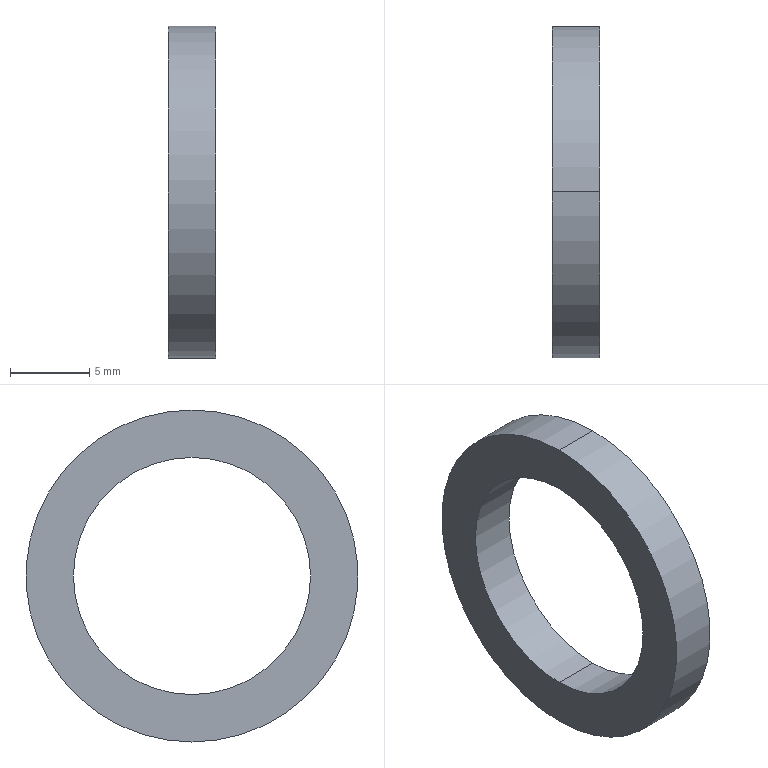Part | SolidWorks | features BaseBody 1 | 1 solid | 6 faces | box 3 x 21 x 21 mm | volume 508.938 mm3 | cylinder 4 | plane 2 | commonest cylinder face diameters 15 x2 21 x2
STEP:
#1=CARTESIAN_POINT('',(3.,0.,10.5));
#2=VERTEX_POINT('',#1);
#3=CARTESIAN_POINT('',(3.,0.,-10.5));
#4=VERTEX_POINT('',#3);
#5=CARTESIAN_POINT('',(3.,0.,0.));
#6=DIRECTION('',(-1.,0.,0.));
#7=DIRECTION('',(0.,0.,1.));
#8=AXIS2_PLACEMENT_3D('',#5,#6,#7);
#9=CIRCLE('',#8,10.5);
#10=EDGE_CURVE('',#2,#4,#9,.T.);
#11=ORIENTED_EDGE('',*,*,#10,.T.);
#12=CARTESIAN_POINT('',(0.,0.,-10.5));
#13=VERTEX_POINT('',#12);
#14=CARTESIAN_POINT('',(3.,0.,-10.5));
#15=DIRECTION('',(-1.,0.,0.));
#16=VECTOR('',#15,1000.);
#17=LINE('',#14,#16);
#18=EDGE_CURVE('',#4,#13,#17,.T.);
#19=ORIENTED_EDGE('',*,*,#18,.T.);
#20=CARTESIAN_POINT('',(0.,0.,10.5));
#21=VERTEX_POINT('',#20);
#22=CARTESIAN_POINT('',(0.,0.,0.));
#23=DIRECTION('',(1.,0.,0.));
#24=DIRECTION('',(0.,0.,1.));
#25=AXIS2_PLACEMENT_3D('',#22,#23,#24);
#26=CIRCLE('',#25,10.5);
#27=EDGE_CURVE('',#13,#21,#26,.T.);
#28=ORIENTED_EDGE('',*,*,#27,.T.);
#29=CARTESIAN_POINT('',(3.,0.,10.5));
#30=DIRECTION('',(-1.,0.,0.));
#31=VECTOR('',#30,1000.);
#32=LINE('',#29,#31);
#33=EDGE_CURVE('',#2,#21,#32,.T.);
#34=ORIENTED_EDGE('',*,*,#33,.F.);
#35=EDGE_LOOP('',(#11,#19,#28,#34));
#36=FACE_OUTER_BOUND('',#35,.T.);
#37=CARTESIAN_POINT('',(3.,0.,0.));
#38=DIRECTION('',(-1.,0.,0.));
#39=DIRECTION('',(0.,0.,1.));
#40=AXIS2_PLACEMENT_3D('',#37,#38,#39);
#41=CYLINDRICAL_SURFACE('',#40,10.5);
#42=ADVANCED_FACE('',(#36),#41,.T.);
#43=CARTESIAN_POINT('',(3.,0.,-7.5));
#44=VERTEX_POINT('',#43);
#45=CARTESIAN_POINT('',(3.,0.,7.5));
#46=VERTEX_POINT('',#45);
#47=CARTESIAN_POINT('',(3.,0.,0.));
#48=DIRECTION('',(-1.,0.,0.));
#49=DIRECTION('',(0.,0.,1.));
#50=AXIS2_PLACEMENT_3D('',#47,#48,#49);
#51=CIRCLE('',#50,7.5);
#52=EDGE_CURVE('',#44,#46,#51,.T.);
#53=ORIENTED_EDGE('',*,*,#52,.F.);
#54=CARTESIAN_POINT('',(0.,0.,-7.5));
#55=VERTEX_POINT('',#54);
#56=CARTESIAN_POINT('',(3.,0.,-7.5));
#57=DIRECTION('',(-1.,0.,0.));
#58=VECTOR('',#57,1000.);
#59=LINE('',#56,#58);
#60=EDGE_CURVE('',#44,#55,#59,.T.);
#61=ORIENTED_EDGE('',*,*,#60,.T.);
#62=CARTESIAN_POINT('',(0.,0.,7.5));
#63=VERTEX_POINT('',#62);
#64=CARTESIAN_POINT('',(0.,0.,0.));
#65=DIRECTION('',(1.,0.,0.));
#66=DIRECTION('',(0.,0.,1.));
#67=AXIS2_PLACEMENT_3D('',#64,#65,#66);
#68=CIRCLE('',#67,7.5);
#69=EDGE_CURVE('',#63,#55,#68,.T.);
#70=ORIENTED_EDGE('',*,*,#69,.F.);
#71=CARTESIAN_POINT('',(3.,0.,7.5));
#72=DIRECTION('',(-1.,0.,0.));
#73=VECTOR('',#72,1000.);
#74=LINE('',#71,#73);
#75=EDGE_CURVE('',#46,#63,#74,.T.);
#76=ORIENTED_EDGE('',*,*,#75,.F.);
#77=EDGE_LOOP('',(#53,#61,#70,#76));
#78=FACE_OUTER_BOUND('',#77,.T.);
#79=CARTESIAN_POINT('',(3.,0.,0.));
#80=DIRECTION('',(-1.,0.,0.));
#81=DIRECTION('',(0.,0.,1.));
#82=AXIS2_PLACEMENT_3D('',#79,#80,#81);
#83=CYLINDRICAL_SURFACE('',#82,7.5);
#84=ADVANCED_FACE('',(#78),#83,.F.);
#85=ORIENTED_EDGE('',*,*,#18,.F.);
#86=CARTESIAN_POINT('',(3.,0.,0.));
#87=DIRECTION('',(-1.,0.,0.));
#88=DIRECTION('',(0.,0.,1.));
#89=AXIS2_PLACEMENT_3D('',#86,#87,#88);
#90=CIRCLE('',#89,10.5);
#91=EDGE_CURVE('',#4,#2,#90,.T.);
#92=ORIENTED_EDGE('',*,*,#91,.T.);
#93=ORIENTED_EDGE('',*,*,#33,.T.);
#94=CARTESIAN_POINT('',(0.,0.,0.));
#95=DIRECTION('',(1.,0.,0.));
#96=DIRECTION('',(0.,0.,1.));
#97=AXIS2_PLACEMENT_3D('',#94,#95,#96);
#98=CIRCLE('',#97,10.5);
#99=EDGE_CURVE('',#21,#13,#98,.T.);
#100=ORIENTED_EDGE('',*,*,#99,.T.);
#101=EDGE_LOOP('',(#85,#92,#93,#100));
#102=FACE_OUTER_BOUND('',#101,.T.);
#103=CARTESIAN_POINT('',(3.,0.,0.));
#104=DIRECTION('',(-1.,0.,0.));
#105=DIRECTION('',(0.,0.,1.));
#106=AXIS2_PLACEMENT_3D('',#103,#104,#105);
#107=CYLINDRICAL_SURFACE('',#106,10.5);
#108=ADVANCED_FACE('',(#102),#107,.T.);
#109=CARTESIAN_POINT('',(3.,0.,0.));
#110=DIRECTION('',(-1.,0.,0.));
#111=DIRECTION('',(0.,0.,1.));
#112=AXIS2_PLACEMENT_3D('',#109,#110,#111);
#113=CIRCLE('',#112,7.5);
#114=EDGE_CURVE('',#46,#44,#113,.T.);
#115=ORIENTED_EDGE('',*,*,#114,.T.);
#116=ORIENTED_EDGE('',*,*,#52,.T.);
#117=EDGE_LOOP('',(#115,#116));
#118=FACE_BOUND('',#117,.T.);
#119=ORIENTED_EDGE('',*,*,#10,.F.);
#120=ORIENTED_EDGE('',*,*,#91,.F.);
#121=EDGE_LOOP('',(#119,#120));
#122=FACE_OUTER_BOUND('',#121,.T.);
#123=CARTESIAN_POINT('',(3.,7.5,0.));
#124=DIRECTION('',(1.,0.,0.));
#125=DIRECTION('',(0.,0.,-1.));
#126=AXIS2_PLACEMENT_3D('',#123,#124,#125);
#127=PLANE('',#126);
#128=ADVANCED_FACE('',(#118,#122),#127,.T.);
#129=ORIENTED_EDGE('',*,*,#99,.F.);
#130=ORIENTED_EDGE('',*,*,#27,.F.);
#131=EDGE_LOOP('',(#129,#130));
#132=FACE_OUTER_BOUND('',#131,.T.);
#133=ORIENTED_EDGE('',*,*,#69,.T.);
#134=CARTESIAN_POINT('',(0.,0.,0.));
#135=DIRECTION('',(1.,0.,0.));
#136=DIRECTION('',(0.,0.,1.));
#137=AXIS2_PLACEMENT_3D('',#134,#135,#136);
#138=CIRCLE('',#137,7.5);
#139=EDGE_CURVE('',#55,#63,#138,.T.);
#140=ORIENTED_EDGE('',*,*,#139,.T.);
#141=EDGE_LOOP('',(#133,#140));
#142=FACE_BOUND('',#141,.T.);
#143=CARTESIAN_POINT('',(0.,10.5,0.));
#144=DIRECTION('',(-1.,0.,0.));
#145=DIRECTION('',(0.,0.,1.));
#146=AXIS2_PLACEMENT_3D('',#143,#144,#145);
#147=PLANE('',#146);
#148=ADVANCED_FACE('',(#132,#142),#147,.T.);
#149=ORIENTED_EDGE('',*,*,#60,.F.);
#150=ORIENTED_EDGE('',*,*,#114,.F.);
#151=ORIENTED_EDGE('',*,*,#75,.T.);
#152=ORIENTED_EDGE('',*,*,#139,.F.);
#153=EDGE_LOOP('',(#149,#150,#151,#152));
#154=FACE_OUTER_BOUND('',#153,.T.);
#155=CARTESIAN_POINT('',(3.,0.,0.));
#156=DIRECTION('',(-1.,0.,0.));
#157=DIRECTION('',(0.,0.,1.));
#158=AXIS2_PLACEMENT_3D('',#155,#156,#157);
#159=CYLINDRICAL_SURFACE('',#158,7.5);
#160=ADVANCED_FACE('',(#154),#159,.F.);
#161=CLOSED_SHELL('',(#42,#84,#108,#128,#148,#160));
#162=MANIFOLD_SOLID_BREP('',#161);
#163=CARTESIAN_POINT('',(0.,0.,0.));
#164=DIRECTION('',(0.,0.,1.));
#165=DIRECTION('',(1.,0.,0.));
#166=AXIS2_PLACEMENT_3D('',#163,#164,#165);
#167=(LENGTH_UNIT()NAMED_UNIT(*)SI_UNIT(.MILLI.,.METRE.));
#168=UNCERTAINTY_MEASURE_WITH_UNIT(LENGTH_MEASURE(0.00001),#167,'','');
#169=(NAMED_UNIT(*)PLANE_ANGLE_UNIT()SI_UNIT($,.RADIAN.));
#170=(NAMED_UNIT(*)SI_UNIT($,.STERADIAN.)SOLID_ANGLE_UNIT());
#171=(GEOMETRIC_REPRESENTATION_CONTEXT(3)GLOBAL_UNCERTAINTY_ASSIGNED_CONTEXT((#168))GLOBAL_UNIT_ASSIGNED_CONTEXT((#167,#169,#170))REPRESENTATION_CONTEXT('',''));
#172=ADVANCED_BREP_SHAPE_REPRESENTATION('',(#162,#166),#171);